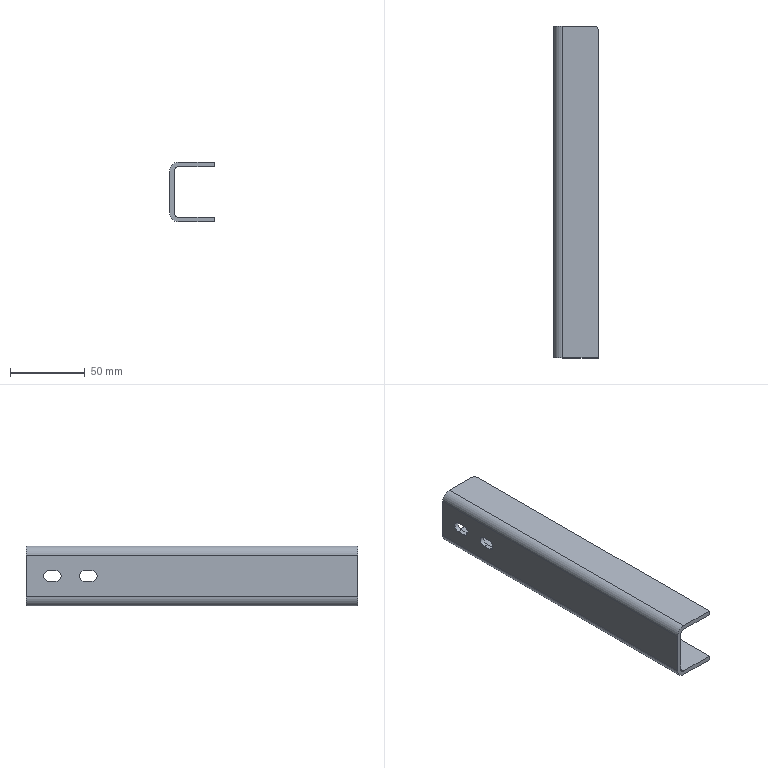Part | NX | features solid 2 | 1 solid | 24 faces | box 30 x 222 x 40 mm | volume 59579 mm3 | plane 14 | cylinder 10 | commonest cylinder face diameters 6 x4 7 x4 12 x2
STEP:
#1=CARTESIAN_POINT('',(340.,-413.,805.));
#2=VERTEX_POINT('',#1);
#3=CARTESIAN_POINT('',(343.,-416.,805.));
#4=VERTEX_POINT('',#3);
#5=CARTESIAN_POINT('',(340.,-416.,805.));
#6=DIRECTION('',(0.,0.,-1.));
#7=DIRECTION('',(-1.,0.,0.));
#8=AXIS2_PLACEMENT_3D('',#5,#6,#7);
#9=CIRCLE('',#8,3.);
#10=EDGE_CURVE('',#2,#4,#9,.T.);
#11=ORIENTED_EDGE('',*,*,#10,.F.);
#12=CARTESIAN_POINT('',(340.,-413.,808.));
#13=VERTEX_POINT('',#12);
#14=CARTESIAN_POINT('',(340.,-413.,802.));
#15=DIRECTION('',(0.,0.,-1.));
#16=VECTOR('',#15,1000.);
#17=LINE('',#14,#16);
#18=EDGE_CURVE('',#13,#2,#17,.T.);
#19=ORIENTED_EDGE('',*,*,#18,.F.);
#20=CARTESIAN_POINT('',(343.,-416.,808.));
#21=VERTEX_POINT('',#20);
#22=CARTESIAN_POINT('',(340.,-416.,808.));
#23=DIRECTION('',(0.,0.,1.));
#24=DIRECTION('',(-1.,0.,0.));
#25=AXIS2_PLACEMENT_3D('',#22,#23,#24);
#26=CIRCLE('',#25,3.);
#27=EDGE_CURVE('',#21,#13,#26,.T.);
#28=ORIENTED_EDGE('',*,*,#27,.F.);
#29=CARTESIAN_POINT('',(343.,-416.,808.));
#30=DIRECTION('',(0.,0.,1.));
#31=VECTOR('',#30,1000.);
#32=LINE('',#29,#31);
#33=EDGE_CURVE('',#4,#21,#32,.T.);
#34=ORIENTED_EDGE('',*,*,#33,.F.);
#35=EDGE_LOOP('',(#11,#19,#28,#34));
#36=FACE_BOUND('',#35,.T.);
#37=CARTESIAN_POINT('',(340.,-416.,808.));
#38=DIRECTION('',(0.,0.,1.));
#39=DIRECTION('',(1.,0.,0.));
#40=AXIS2_PLACEMENT_3D('',#37,#38,#39);
#41=CYLINDRICAL_SURFACE('',#40,3.);
#42=ADVANCED_FACE('',(#36),#41,.T.);
#43=CARTESIAN_POINT('',(343.,-416.,771.));
#44=VERTEX_POINT('',#43);
#45=CARTESIAN_POINT('',(340.,-413.,771.));
#46=VERTEX_POINT('',#45);
#47=CARTESIAN_POINT('',(340.,-416.,771.));
#48=DIRECTION('',(0.,0.,1.));
#49=DIRECTION('',(1.,0.,0.));
#50=AXIS2_PLACEMENT_3D('',#47,#48,#49);
#51=CIRCLE('',#50,3.);
#52=EDGE_CURVE('',#44,#46,#51,.T.);
#53=ORIENTED_EDGE('',*,*,#52,.F.);
#54=CARTESIAN_POINT('',(343.,-416.,768.));
#55=VERTEX_POINT('',#54);
#56=CARTESIAN_POINT('',(343.,-416.,768.));
#57=DIRECTION('',(0.,0.,1.));
#58=VECTOR('',#57,1000.);
#59=LINE('',#56,#58);
#60=EDGE_CURVE('',#55,#44,#59,.T.);
#61=ORIENTED_EDGE('',*,*,#60,.F.);
#62=CARTESIAN_POINT('',(340.,-413.,768.));
#63=VERTEX_POINT('',#62);
#64=CARTESIAN_POINT('',(340.,-416.,768.));
#65=DIRECTION('',(0.,0.,-1.));
#66=DIRECTION('',(1.,0.,0.));
#67=AXIS2_PLACEMENT_3D('',#64,#65,#66);
#68=CIRCLE('',#67,3.);
#69=EDGE_CURVE('',#63,#55,#68,.T.);
#70=ORIENTED_EDGE('',*,*,#69,.F.);
#71=CARTESIAN_POINT('',(340.,-413.,802.));
#72=DIRECTION('',(0.,0.,-1.));
#73=VECTOR('',#72,1000.);
#74=LINE('',#71,#73);
#75=EDGE_CURVE('',#46,#63,#74,.T.);
#76=ORIENTED_EDGE('',*,*,#75,.F.);
#77=EDGE_LOOP('',(#53,#61,#70,#76));
#78=FACE_BOUND('',#77,.T.);
#79=CARTESIAN_POINT('',(340.,-416.,802.));
#80=DIRECTION('',(0.,0.,1.));
#81=DIRECTION('',(1.,0.,0.));
#82=AXIS2_PLACEMENT_3D('',#79,#80,#81);
#83=CYLINDRICAL_SURFACE('',#82,3.);
#84=ADVANCED_FACE('',(#78),#83,.T.);
#85=CARTESIAN_POINT('',(313.,-428.,791.5));
#86=VERTEX_POINT('',#85);
#87=CARTESIAN_POINT('',(316.,-428.,791.5));
#88=VERTEX_POINT('',#87);
#89=CARTESIAN_POINT('',(88.439,-428.,791.5));
#90=DIRECTION('',(1.,0.,0.));
#91=VECTOR('',#90,1000.);
#92=LINE('',#89,#91);
#93=EDGE_CURVE('',#86,#88,#92,.T.);
#94=ORIENTED_EDGE('',*,*,#93,.T.);
#95=CARTESIAN_POINT('',(316.,-433.,791.5));
#96=VERTEX_POINT('',#95);
#97=CARTESIAN_POINT('',(316.,-428.,791.5));
#98=DIRECTION('',(0.,-1.,0.));
#99=VECTOR('',#98,1000.);
#100=LINE('',#97,#99);
#101=EDGE_CURVE('',#88,#96,#100,.T.);
#102=ORIENTED_EDGE('',*,*,#101,.T.);
#103=CARTESIAN_POINT('',(313.,-433.,791.5));
#104=VERTEX_POINT('',#103);
#105=CARTESIAN_POINT('',(88.439,-433.,791.5));
#106=DIRECTION('',(1.,0.,0.));
#107=VECTOR('',#106,1000.);
#108=LINE('',#105,#107);
#109=EDGE_CURVE('',#104,#96,#108,.T.);
#110=ORIENTED_EDGE('',*,*,#109,.F.);
#111=CARTESIAN_POINT('',(313.,-635.,791.5));
#112=DIRECTION('',(0.,-1.,0.));
#113=VECTOR('',#112,1000.);
#114=LINE('',#111,#113);
#115=EDGE_CURVE('',#86,#104,#114,.T.);
#116=ORIENTED_EDGE('',*,*,#115,.F.);
#117=EDGE_LOOP('',(#94,#102,#110,#116));
#118=FACE_BOUND('',#117,.T.);
#119=CARTESIAN_POINT('',(88.439,-428.,791.5));
#120=DIRECTION('',(0.,0.,1.));
#121=DIRECTION('',(0.,-1.,0.));
#122=AXIS2_PLACEMENT_3D('',#119,#120,#121);
#123=PLANE('',#122);
#124=ADVANCED_FACE('',(#118),#123,.F.);
#125=CARTESIAN_POINT('',(313.,-428.,784.5));
#126=VERTEX_POINT('',#125);
#127=CARTESIAN_POINT('',(316.,-428.,784.5));
#128=VERTEX_POINT('',#127);
#129=CARTESIAN_POINT('',(88.439,-428.,784.5));
#130=DIRECTION('',(1.,0.,0.));
#131=VECTOR('',#130,1000.);
#132=LINE('',#129,#131);
#133=EDGE_CURVE('',#126,#128,#132,.T.);
#134=ORIENTED_EDGE('',*,*,#133,.T.);
#135=CARTESIAN_POINT('',(316.,-428.,788.));
#136=DIRECTION('',(1.,0.,0.));
#137=DIRECTION('',(0.,-1.,0.));
#138=AXIS2_PLACEMENT_3D('',#135,#136,#137);
#139=CIRCLE('',#138,3.5);
#140=EDGE_CURVE('',#128,#88,#139,.T.);
#141=ORIENTED_EDGE('',*,*,#140,.T.);
#142=ORIENTED_EDGE('',*,*,#93,.F.);
#143=CARTESIAN_POINT('',(313.,-428.,788.));
#144=DIRECTION('',(1.,0.,0.));
#145=DIRECTION('',(0.,0.,-1.));
#146=AXIS2_PLACEMENT_3D('',#143,#144,#145);
#147=CIRCLE('',#146,3.5);
#148=EDGE_CURVE('',#126,#86,#147,.T.);
#149=ORIENTED_EDGE('',*,*,#148,.F.);
#150=EDGE_LOOP('',(#134,#141,#142,#149));
#151=FACE_BOUND('',#150,.T.);
#152=CARTESIAN_POINT('',(88.439,-428.,788.));
#153=DIRECTION('',(1.,0.,0.));
#154=DIRECTION('',(0.,0.,-1.));
#155=AXIS2_PLACEMENT_3D('',#152,#153,#154);
#156=CYLINDRICAL_SURFACE('',#155,3.5);
#157=ADVANCED_FACE('',(#151),#156,.F.);
#158=CARTESIAN_POINT('',(313.,-433.,784.5));
#159=VERTEX_POINT('',#158);
#160=CARTESIAN_POINT('',(316.,-433.,784.5));
#161=VERTEX_POINT('',#160);
#162=CARTESIAN_POINT('',(88.439,-433.,784.5));
#163=DIRECTION('',(1.,0.,0.));
#164=VECTOR('',#163,1000.);
#165=LINE('',#162,#164);
#166=EDGE_CURVE('',#159,#161,#165,.T.);
#167=ORIENTED_EDGE('',*,*,#166,.T.);
#168=CARTESIAN_POINT('',(316.,-428.,784.5));
#169=DIRECTION('',(0.,1.,0.));
#170=VECTOR('',#169,1000.);
#171=LINE('',#168,#170);
#172=EDGE_CURVE('',#161,#128,#171,.T.);
#173=ORIENTED_EDGE('',*,*,#172,.T.);
#174=ORIENTED_EDGE('',*,*,#133,.F.);
#175=CARTESIAN_POINT('',(313.,-635.,784.5));
#176=DIRECTION('',(0.,1.,0.));
#177=VECTOR('',#176,1000.);
#178=LINE('',#175,#177);
#179=EDGE_CURVE('',#159,#126,#178,.T.);
#180=ORIENTED_EDGE('',*,*,#179,.F.);
#181=EDGE_LOOP('',(#167,#173,#174,#180));
#182=FACE_BOUND('',#181,.T.);
#183=CARTESIAN_POINT('',(88.439,-428.,784.5));
#184=DIRECTION('',(0.,0.,-1.));
#185=DIRECTION('',(-1.,0.,0.));
#186=AXIS2_PLACEMENT_3D('',#183,#184,#185);
#187=PLANE('',#186);
#188=ADVANCED_FACE('',(#182),#187,.F.);
#189=ORIENTED_EDGE('',*,*,#109,.T.);
#190=CARTESIAN_POINT('',(316.,-433.,788.));
#191=DIRECTION('',(1.,0.,0.));
#192=DIRECTION('',(0.,1.,0.));
#193=AXIS2_PLACEMENT_3D('',#190,#191,#192);
#194=CIRCLE('',#193,3.5);
#195=EDGE_CURVE('',#96,#161,#194,.T.);
#196=ORIENTED_EDGE('',*,*,#195,.T.);
#197=ORIENTED_EDGE('',*,*,#166,.F.);
#198=CARTESIAN_POINT('',(313.,-433.,788.));
#199=DIRECTION('',(1.,0.,0.));
#200=DIRECTION('',(0.,0.,-1.));
#201=AXIS2_PLACEMENT_3D('',#198,#199,#200);
#202=CIRCLE('',#201,3.5);
#203=EDGE_CURVE('',#104,#159,#202,.T.);
#204=ORIENTED_EDGE('',*,*,#203,.F.);
#205=EDGE_LOOP('',(#189,#196,#197,#204));
#206=FACE_BOUND('',#205,.T.);
#207=CARTESIAN_POINT('',(88.439,-433.,788.));
#208=DIRECTION('',(1.,0.,0.));
#209=DIRECTION('',(0.,0.,-1.));
#210=AXIS2_PLACEMENT_3D('',#207,#208,#209);
#211=CYLINDRICAL_SURFACE('',#210,3.5);
#212=ADVANCED_FACE('',(#206),#211,.F.);
#213=CARTESIAN_POINT('',(313.,-452.,791.5));
#214=VERTEX_POINT('',#213);
#215=CARTESIAN_POINT('',(316.,-452.,791.5));
#216=VERTEX_POINT('',#215);
#217=CARTESIAN_POINT('',(88.439,-452.,791.5));
#218=DIRECTION('',(1.,0.,0.));
#219=VECTOR('',#218,1000.);
#220=LINE('',#217,#219);
#221=EDGE_CURVE('',#214,#216,#220,.T.);
#222=ORIENTED_EDGE('',*,*,#221,.T.);
#223=CARTESIAN_POINT('',(316.,-457.,791.5));
#224=VERTEX_POINT('',#223);
#225=CARTESIAN_POINT('',(316.,-452.,791.5));
#226=DIRECTION('',(0.,-1.,0.));
#227=VECTOR('',#226,1000.);
#228=LINE('',#225,#227);
#229=EDGE_CURVE('',#216,#224,#228,.T.);
#230=ORIENTED_EDGE('',*,*,#229,.T.);
#231=CARTESIAN_POINT('',(313.,-457.,791.5));
#232=VERTEX_POINT('',#231);
#233=CARTESIAN_POINT('',(88.439,-457.,791.5));
#234=DIRECTION('',(1.,0.,0.));
#235=VECTOR('',#234,1000.);
#236=LINE('',#233,#235);
#237=EDGE_CURVE('',#232,#224,#236,.T.);
#238=ORIENTED_EDGE('',*,*,#237,.F.);
#239=CARTESIAN_POINT('',(313.,-635.,791.5));
#240=DIRECTION('',(0.,-1.,0.));
#241=VECTOR('',#240,1000.);
#242=LINE('',#239,#241);
#243=EDGE_CURVE('',#214,#232,#242,.T.);
#244=ORIENTED_EDGE('',*,*,#243,.F.);
#245=EDGE_LOOP('',(#222,#230,#238,#244));
#246=FACE_BOUND('',#245,.T.);
#247=CARTESIAN_POINT('',(88.439,-452.,791.5));
#248=DIRECTION('',(0.,0.,1.));
#249=DIRECTION('',(0.,-1.,0.));
#250=AXIS2_PLACEMENT_3D('',#247,#248,#249);
#251=PLANE('',#250);
#252=ADVANCED_FACE('',(#246),#251,.F.);
#253=CARTESIAN_POINT('',(313.,-452.,784.5));
#254=VERTEX_POINT('',#253);
#255=CARTESIAN_POINT('',(316.,-452.,784.5));
#256=VERTEX_POINT('',#255);
#257=CARTESIAN_POINT('',(88.439,-452.,784.5));
#258=DIRECTION('',(1.,0.,0.));
#259=VECTOR('',#258,1000.);
#260=LINE('',#257,#259);
#261=EDGE_CURVE('',#254,#256,#260,.T.);
#262=ORIENTED_EDGE('',*,*,#261,.T.);
#263=CARTESIAN_POINT('',(316.,-452.,788.));
#264=DIRECTION('',(1.,0.,0.));
#265=DIRECTION('',(0.,-1.,0.));
#266=AXIS2_PLACEMENT_3D('',#263,#264,#265);
#267=CIRCLE('',#266,3.5);
#268=EDGE_CURVE('',#256,#216,#267,.T.);
#269=ORIENTED_EDGE('',*,*,#268,.T.);
#270=ORIENTED_EDGE('',*,*,#221,.F.);
#271=CARTESIAN_POINT('',(313.,-452.,788.));
#272=DIRECTION('',(1.,0.,0.));
#273=DIRECTION('',(0.,0.,-1.));
#274=AXIS2_PLACEMENT_3D('',#271,#272,#273);
#275=CIRCLE('',#274,3.5);
#276=EDGE_CURVE('',#254,#214,#275,.T.);
#277=ORIENTED_EDGE('',*,*,#276,.F.);
#278=EDGE_LOOP('',(#262,#269,#270,#277));
#279=FACE_BOUND('',#278,.T.);
#280=CARTESIAN_POINT('',(88.439,-452.,788.));
#281=DIRECTION('',(1.,0.,0.));
#282=DIRECTION('',(0.,0.,-1.));
#283=AXIS2_PLACEMENT_3D('',#280,#281,#282);
#284=CYLINDRICAL_SURFACE('',#283,3.5);
#285=ADVANCED_FACE('',(#279),#284,.F.);
#286=CARTESIAN_POINT('',(313.,-457.,784.5));
#287=VERTEX_POINT('',#286);
#288=CARTESIAN_POINT('',(316.,-457.,784.5));
#289=VERTEX_POINT('',#288);
#290=CARTESIAN_POINT('',(88.439,-457.,784.5));
#291=DIRECTION('',(1.,0.,0.));
#292=VECTOR('',#291,1000.);
#293=LINE('',#290,#292);
#294=EDGE_CURVE('',#287,#289,#293,.T.);
#295=ORIENTED_EDGE('',*,*,#294,.T.);
#296=CARTESIAN_POINT('',(316.,-452.,784.5));
#297=DIRECTION('',(0.,1.,0.));
#298=VECTOR('',#297,1000.);
#299=LINE('',#296,#298);
#300=EDGE_CURVE('',#289,#256,#299,.T.);
#301=ORIENTED_EDGE('',*,*,#300,.T.);
#302=ORIENTED_EDGE('',*,*,#261,.F.);
#303=CARTESIAN_POINT('',(313.,-635.,784.5));
#304=DIRECTION('',(0.,1.,0.));
#305=VECTOR('',#304,1000.);
#306=LINE('',#303,#305);
#307=EDGE_CURVE('',#287,#254,#306,.T.);
#308=ORIENTED_EDGE('',*,*,#307,.F.);
#309=EDGE_LOOP('',(#295,#301,#302,#308));
#310=FACE_BOUND('',#309,.T.);
#311=CARTESIAN_POINT('',(88.439,-452.,784.5));
#312=DIRECTION('',(0.,0.,-1.));
#313=DIRECTION('',(-1.,0.,0.));
#314=AXIS2_PLACEMENT_3D('',#311,#312,#313);
#315=PLANE('',#314);
#316=ADVANCED_FACE('',(#310),#315,.F.);
#317=ORIENTED_EDGE('',*,*,#237,.T.);
#318=CARTESIAN_POINT('',(316.,-457.,788.));
#319=DIRECTION('',(1.,0.,0.));
#320=DIRECTION('',(0.,1.,0.));
#321=AXIS2_PLACEMENT_3D('',#318,#319,#320);
#322=CIRCLE('',#321,3.5);
#323=EDGE_CURVE('',#224,#289,#322,.T.);
#324=ORIENTED_EDGE('',*,*,#323,.T.);
#325=ORIENTED_EDGE('',*,*,#294,.F.);
#326=CARTESIAN_POINT('',(313.,-457.,788.));
#327=DIRECTION('',(1.,0.,0.));
#328=DIRECTION('',(0.,0.,-1.));
#329=AXIS2_PLACEMENT_3D('',#326,#327,#328);
#330=CIRCLE('',#329,3.5);
#331=EDGE_CURVE('',#232,#287,#330,.T.);
#332=ORIENTED_EDGE('',*,*,#331,.F.);
#333=EDGE_LOOP('',(#317,#324,#325,#332));
#334=FACE_BOUND('',#333,.T.);
#335=CARTESIAN_POINT('',(88.439,-457.,788.));
#336=DIRECTION('',(1.,0.,0.));
#337=DIRECTION('',(0.,0.,-1.));
#338=AXIS2_PLACEMENT_3D('',#335,#336,#337);
#339=CYLINDRICAL_SURFACE('',#338,3.5);
#340=ADVANCED_FACE('',(#334),#339,.F.);
#341=CARTESIAN_POINT('',(343.,-635.,771.));
#342=VERTEX_POINT('',#341);
#343=CARTESIAN_POINT('',(343.,-635.,771.));
#344=DIRECTION('',(0.,1.,0.));
#345=VECTOR('',#344,1000.);
#346=LINE('',#343,#345);
#347=EDGE_CURVE('',#342,#44,#346,.T.);
#348=ORIENTED_EDGE('',*,*,#347,.T.);
#349=ORIENTED_EDGE('',*,*,#52,.T.);
#350=CARTESIAN_POINT('',(319.,-413.,771.));
#351=VERTEX_POINT('',#350);
#352=CARTESIAN_POINT('',(313.,-413.,771.));
#353=DIRECTION('',(1.,0.,0.));
#354=VECTOR('',#353,1000.);
#355=LINE('',#352,#354);
#356=EDGE_CURVE('',#351,#46,#355,.T.);
#357=ORIENTED_EDGE('',*,*,#356,.F.);
#358=CARTESIAN_POINT('',(319.,-635.,771.));
#359=VERTEX_POINT('',#358);
#360=CARTESIAN_POINT('',(319.,-635.,771.));
#361=DIRECTION('',(0.,1.,0.));
#362=VECTOR('',#361,1000.);
#363=LINE('',#360,#362);
#364=EDGE_CURVE('',#359,#351,#363,.T.);
#365=ORIENTED_EDGE('',*,*,#364,.F.);
#366=CARTESIAN_POINT('',(313.,-635.,771.));
#367=DIRECTION('',(1.,0.,0.));
#368=VECTOR('',#367,1000.);
#369=LINE('',#366,#368);
#370=EDGE_CURVE('',#359,#342,#369,.T.);
#371=ORIENTED_EDGE('',*,*,#370,.T.);
#372=EDGE_LOOP('',(#348,#349,#357,#365,#371));
#373=FACE_BOUND('',#372,.T.);
#374=CARTESIAN_POINT('',(313.,-635.,771.));
#375=DIRECTION('',(0.,0.,1.));
#376=DIRECTION('',(1.,0.,0.));
#377=AXIS2_PLACEMENT_3D('',#374,#375,#376);
#378=PLANE('',#377);
#379=ADVANCED_FACE('',(#373),#378,.T.);
#380=CARTESIAN_POINT('',(316.,-413.,774.));
#381=VERTEX_POINT('',#380);
#382=CARTESIAN_POINT('',(319.,-413.,774.));
#383=DIRECTION('',(0.,-1.,0.));
#384=DIRECTION('',(0.,0.,1.));
#385=AXIS2_PLACEMENT_3D('',#382,#383,#384);
#386=CIRCLE('',#385,3.);
#387=EDGE_CURVE('',#381,#351,#386,.T.);
#388=ORIENTED_EDGE('',*,*,#387,.F.);
#389=CARTESIAN_POINT('',(316.,-635.,774.));
#390=VERTEX_POINT('',#389);
#391=CARTESIAN_POINT('',(316.,-635.,774.));
#392=DIRECTION('',(0.,1.,0.));
#393=VECTOR('',#392,1000.);
#394=LINE('',#391,#393);
#395=EDGE_CURVE('',#390,#381,#394,.T.);
#396=ORIENTED_EDGE('',*,*,#395,.F.);
#397=CARTESIAN_POINT('',(319.,-635.,774.));
#398=DIRECTION('',(0.,-1.,0.));
#399=DIRECTION('',(0.,0.,1.));
#400=AXIS2_PLACEMENT_3D('',#397,#398,#399);
#401=CIRCLE('',#400,3.);
#402=EDGE_CURVE('',#390,#359,#401,.T.);
#403=ORIENTED_EDGE('',*,*,#402,.T.);
#404=ORIENTED_EDGE('',*,*,#364,.T.);
#405=EDGE_LOOP('',(#388,#396,#403,#404));
#406=FACE_BOUND('',#405,.T.);
#407=CARTESIAN_POINT('',(319.,-635.,774.));
#408=DIRECTION('',(0.,1.,0.));
#409=DIRECTION('',(0.,0.,1.));
#410=AXIS2_PLACEMENT_3D('',#407,#408,#409);
#411=CYLINDRICAL_SURFACE('',#410,3.);
#412=ADVANCED_FACE('',(#406),#411,.F.);
#413=ORIENTED_EDGE('',*,*,#323,.F.);
#414=ORIENTED_EDGE('',*,*,#229,.F.);
#415=ORIENTED_EDGE('',*,*,#268,.F.);
#416=ORIENTED_EDGE('',*,*,#300,.F.);
#417=EDGE_LOOP('',(#413,#414,#415,#416));
#418=FACE_BOUND('',#417,.T.);
#419=ORIENTED_EDGE('',*,*,#195,.F.);
#420=ORIENTED_EDGE('',*,*,#101,.F.);
#421=ORIENTED_EDGE('',*,*,#140,.F.);
#422=ORIENTED_EDGE('',*,*,#172,.F.);
#423=EDGE_LOOP('',(#419,#420,#421,#422));
#424=FACE_BOUND('',#423,.T.);
#425=CARTESIAN_POINT('',(316.,-413.,802.));
#426=VERTEX_POINT('',#425);
#427=CARTESIAN_POINT('',(316.,-413.,808.));
#428=DIRECTION('',(0.,0.,-1.));
#429=VECTOR('',#428,1000.);
#430=LINE('',#427,#429);
#431=EDGE_CURVE('',#426,#381,#430,.T.);
#432=ORIENTED_EDGE('',*,*,#431,.F.);
#433=CARTESIAN_POINT('',(316.,-635.,802.));
#434=VERTEX_POINT('',#433);
#435=CARTESIAN_POINT('',(316.,-635.,802.));
#436=DIRECTION('',(0.,1.,0.));
#437=VECTOR('',#436,1000.);
#438=LINE('',#435,#437);
#439=EDGE_CURVE('',#434,#426,#438,.T.);
#440=ORIENTED_EDGE('',*,*,#439,.F.);
#441=CARTESIAN_POINT('',(316.,-635.,808.));
#442=DIRECTION('',(0.,0.,-1.));
#443=VECTOR('',#442,1000.);
#444=LINE('',#441,#443);
#445=EDGE_CURVE('',#434,#390,#444,.T.);
#446=ORIENTED_EDGE('',*,*,#445,.T.);
#447=ORIENTED_EDGE('',*,*,#395,.T.);
#448=EDGE_LOOP('',(#432,#440,#446,#447));
#449=FACE_BOUND('',#448,.T.);
#450=CARTESIAN_POINT('',(316.,-635.,808.));
#451=DIRECTION('',(1.,0.,0.));
#452=DIRECTION('',(0.,1.,0.));
#453=AXIS2_PLACEMENT_3D('',#450,#451,#452);
#454=PLANE('',#453);
#455=ADVANCED_FACE('',(#418,#424,#449),#454,.T.);
#456=CARTESIAN_POINT('',(319.,-413.,805.));
#457=VERTEX_POINT('',#456);
#458=CARTESIAN_POINT('',(319.,-413.,802.));
#459=DIRECTION('',(0.,-1.,0.));
#460=DIRECTION('',(0.,0.,1.));
#461=AXIS2_PLACEMENT_3D('',#458,#459,#460);
#462=CIRCLE('',#461,3.);
#463=EDGE_CURVE('',#457,#426,#462,.T.);
#464=ORIENTED_EDGE('',*,*,#463,.F.);
#465=CARTESIAN_POINT('',(319.,-635.,805.));
#466=VERTEX_POINT('',#465);
#467=CARTESIAN_POINT('',(319.,-635.,805.));
#468=DIRECTION('',(0.,1.,0.));
#469=VECTOR('',#468,1000.);
#470=LINE('',#467,#469);
#471=EDGE_CURVE('',#466,#457,#470,.T.);
#472=ORIENTED_EDGE('',*,*,#471,.F.);
#473=CARTESIAN_POINT('',(319.,-635.,802.));
#474=DIRECTION('',(0.,-1.,0.));
#475=DIRECTION('',(0.,0.,1.));
#476=AXIS2_PLACEMENT_3D('',#473,#474,#475);
#477=CIRCLE('',#476,3.);
#478=EDGE_CURVE('',#466,#434,#477,.T.);
#479=ORIENTED_EDGE('',*,*,#478,.T.);
#480=ORIENTED_EDGE('',*,*,#439,.T.);
#481=EDGE_LOOP('',(#464,#472,#479,#480));
#482=FACE_BOUND('',#481,.T.);
#483=CARTESIAN_POINT('',(319.,-635.,802.));
#484=DIRECTION('',(0.,1.,0.));
#485=DIRECTION('',(0.,0.,1.));
#486=AXIS2_PLACEMENT_3D('',#483,#484,#485);
#487=CYLINDRICAL_SURFACE('',#486,3.);
#488=ADVANCED_FACE('',(#482),#487,.F.);
#489=CARTESIAN_POINT('',(343.,-413.,805.));
#490=DIRECTION('',(-1.,0.,0.));
#491=VECTOR('',#490,1000.);
#492=LINE('',#489,#491);
#493=EDGE_CURVE('',#2,#457,#492,.T.);
#494=ORIENTED_EDGE('',*,*,#493,.F.);
#495=ORIENTED_EDGE('',*,*,#10,.T.);
#496=CARTESIAN_POINT('',(343.,-635.,805.));
#497=VERTEX_POINT('',#496);
#498=CARTESIAN_POINT('',(343.,-635.,805.));
#499=DIRECTION('',(0.,1.,0.));
#500=VECTOR('',#499,1000.);
#501=LINE('',#498,#500);
#502=EDGE_CURVE('',#497,#4,#501,.T.);
#503=ORIENTED_EDGE('',*,*,#502,.F.);
#504=CARTESIAN_POINT('',(343.,-635.,805.));
#505=DIRECTION('',(-1.,0.,0.));
#506=VECTOR('',#505,1000.);
#507=LINE('',#504,#506);
#508=EDGE_CURVE('',#497,#466,#507,.T.);
#509=ORIENTED_EDGE('',*,*,#508,.T.);
#510=ORIENTED_EDGE('',*,*,#471,.T.);
#511=EDGE_LOOP('',(#494,#495,#503,#509,#510));
#512=FACE_BOUND('',#511,.T.);
#513=CARTESIAN_POINT('',(343.,-635.,805.));
#514=DIRECTION('',(0.,0.,-1.));
#515=DIRECTION('',(0.,-1.,0.));
#516=AXIS2_PLACEMENT_3D('',#513,#514,#515);
#517=PLANE('',#516);
#518=ADVANCED_FACE('',(#512),#517,.T.);
#519=CARTESIAN_POINT('',(319.,-413.,768.));
#520=VERTEX_POINT('',#519);
#521=CARTESIAN_POINT('',(313.,-413.,768.));
#522=DIRECTION('',(1.,0.,0.));
#523=VECTOR('',#522,1000.);
#524=LINE('',#521,#523);
#525=EDGE_CURVE('',#520,#63,#524,.T.);
#526=ORIENTED_EDGE('',*,*,#525,.T.);
#527=ORIENTED_EDGE('',*,*,#69,.T.);
#528=CARTESIAN_POINT('',(343.,-635.,768.));
#529=VERTEX_POINT('',#528);
#530=CARTESIAN_POINT('',(343.,-635.,768.));
#531=DIRECTION('',(0.,1.,0.));
#532=VECTOR('',#531,1000.);
#533=LINE('',#530,#532);
#534=EDGE_CURVE('',#529,#55,#533,.T.);
#535=ORIENTED_EDGE('',*,*,#534,.F.);
#536=CARTESIAN_POINT('',(319.,-635.,768.));
#537=VERTEX_POINT('',#536);
#538=CARTESIAN_POINT('',(313.,-635.,768.));
#539=DIRECTION('',(1.,0.,0.));
#540=VECTOR('',#539,1000.);
#541=LINE('',#538,#540);
#542=EDGE_CURVE('',#537,#529,#541,.T.);
#543=ORIENTED_EDGE('',*,*,#542,.F.);
#544=CARTESIAN_POINT('',(319.,-635.,768.));
#545=DIRECTION('',(0.,1.,0.));
#546=VECTOR('',#545,1000.);
#547=LINE('',#544,#546);
#548=EDGE_CURVE('',#537,#520,#547,.T.);
#549=ORIENTED_EDGE('',*,*,#548,.T.);
#550=EDGE_LOOP('',(#526,#527,#535,#543,#549));
#551=FACE_BOUND('',#550,.T.);
#552=CARTESIAN_POINT('',(313.,-635.,768.));
#553=DIRECTION('',(0.,0.,1.));
#554=DIRECTION('',(1.,0.,0.));
#555=AXIS2_PLACEMENT_3D('',#552,#553,#554);
#556=PLANE('',#555);
#557=ADVANCED_FACE('',(#551),#556,.F.);
#558=CARTESIAN_POINT('',(313.,-413.,774.));
#559=VERTEX_POINT('',#558);
#560=CARTESIAN_POINT('',(319.,-413.,774.));
#561=DIRECTION('',(0.,-1.,0.));
#562=DIRECTION('',(0.,0.,1.));
#563=AXIS2_PLACEMENT_3D('',#560,#561,#562);
#564=CIRCLE('',#563,6.);
#565=EDGE_CURVE('',#559,#520,#564,.T.);
#566=ORIENTED_EDGE('',*,*,#565,.T.);
#567=ORIENTED_EDGE('',*,*,#548,.F.);
#568=CARTESIAN_POINT('',(313.,-635.,774.));
#569=VERTEX_POINT('',#568);
#570=CARTESIAN_POINT('',(319.,-635.,774.));
#571=DIRECTION('',(0.,-1.,0.));
#572=DIRECTION('',(0.,0.,1.));
#573=AXIS2_PLACEMENT_3D('',#570,#571,#572);
#574=CIRCLE('',#573,6.);
#575=EDGE_CURVE('',#569,#537,#574,.T.);
#576=ORIENTED_EDGE('',*,*,#575,.F.);
#577=CARTESIAN_POINT('',(313.,-635.,774.));
#578=DIRECTION('',(0.,1.,0.));
#579=VECTOR('',#578,1000.);
#580=LINE('',#577,#579);
#581=EDGE_CURVE('',#569,#559,#580,.T.);
#582=ORIENTED_EDGE('',*,*,#581,.T.);
#583=EDGE_LOOP('',(#566,#567,#576,#582));
#584=FACE_BOUND('',#583,.T.);
#585=CARTESIAN_POINT('',(319.,-635.,774.));
#586=DIRECTION('',(0.,1.,0.));
#587=DIRECTION('',(0.,0.,1.));
#588=AXIS2_PLACEMENT_3D('',#585,#586,#587);
#589=CYLINDRICAL_SURFACE('',#588,6.);
#590=ADVANCED_FACE('',(#584),#589,.T.);
#591=ORIENTED_EDGE('',*,*,#243,.T.);
#592=ORIENTED_EDGE('',*,*,#331,.T.);
#593=ORIENTED_EDGE('',*,*,#307,.T.);
#594=ORIENTED_EDGE('',*,*,#276,.T.);
#595=EDGE_LOOP('',(#591,#592,#593,#594));
#596=FACE_BOUND('',#595,.T.);
#597=ORIENTED_EDGE('',*,*,#115,.T.);
#598=ORIENTED_EDGE('',*,*,#203,.T.);
#599=ORIENTED_EDGE('',*,*,#179,.T.);
#600=ORIENTED_EDGE('',*,*,#148,.T.);
#601=EDGE_LOOP('',(#597,#598,#599,#600));
#602=FACE_BOUND('',#601,.T.);
#603=CARTESIAN_POINT('',(313.,-413.,802.));
#604=VERTEX_POINT('',#603);
#605=CARTESIAN_POINT('',(313.,-413.,808.));
#606=DIRECTION('',(0.,0.,-1.));
#607=VECTOR('',#606,1000.);
#608=LINE('',#605,#607);
#609=EDGE_CURVE('',#604,#559,#608,.T.);
#610=ORIENTED_EDGE('',*,*,#609,.T.);
#611=ORIENTED_EDGE('',*,*,#581,.F.);
#612=CARTESIAN_POINT('',(313.,-635.,802.));
#613=VERTEX_POINT('',#612);
#614=CARTESIAN_POINT('',(313.,-635.,808.));
#615=DIRECTION('',(0.,0.,-1.));
#616=VECTOR('',#615,1000.);
#617=LINE('',#614,#616);
#618=EDGE_CURVE('',#613,#569,#617,.T.);
#619=ORIENTED_EDGE('',*,*,#618,.F.);
#620=CARTESIAN_POINT('',(313.,-635.,802.));
#621=DIRECTION('',(0.,1.,0.));
#622=VECTOR('',#621,1000.);
#623=LINE('',#620,#622);
#624=EDGE_CURVE('',#613,#604,#623,.T.);
#625=ORIENTED_EDGE('',*,*,#624,.T.);
#626=EDGE_LOOP('',(#610,#611,#619,#625));
#627=FACE_BOUND('',#626,.T.);
#628=CARTESIAN_POINT('',(313.,-635.,808.));
#629=DIRECTION('',(1.,0.,0.));
#630=DIRECTION('',(0.,1.,0.));
#631=AXIS2_PLACEMENT_3D('',#628,#629,#630);
#632=PLANE('',#631);
#633=ADVANCED_FACE('',(#596,#602,#627),#632,.F.);
#634=CARTESIAN_POINT('',(319.,-413.,808.));
#635=VERTEX_POINT('',#634);
#636=CARTESIAN_POINT('',(319.,-413.,802.));
#637=DIRECTION('',(0.,-1.,0.));
#638=DIRECTION('',(0.,0.,1.));
#639=AXIS2_PLACEMENT_3D('',#636,#637,#638);
#640=CIRCLE('',#639,6.);
#641=EDGE_CURVE('',#635,#604,#640,.T.);
#642=ORIENTED_EDGE('',*,*,#641,.T.);
#643=ORIENTED_EDGE('',*,*,#624,.F.);
#644=CARTESIAN_POINT('',(319.,-635.,808.));
#645=VERTEX_POINT('',#644);
#646=CARTESIAN_POINT('',(319.,-635.,802.));
#647=DIRECTION('',(0.,-1.,0.));
#648=DIRECTION('',(0.,0.,1.));
#649=AXIS2_PLACEMENT_3D('',#646,#647,#648);
#650=CIRCLE('',#649,6.);
#651=EDGE_CURVE('',#645,#613,#650,.T.);
#652=ORIENTED_EDGE('',*,*,#651,.F.);
#653=CARTESIAN_POINT('',(319.,-635.,808.));
#654=DIRECTION('',(0.,1.,0.));
#655=VECTOR('',#654,1000.);
#656=LINE('',#653,#655);
#657=EDGE_CURVE('',#645,#635,#656,.T.);
#658=ORIENTED_EDGE('',*,*,#657,.T.);
#659=EDGE_LOOP('',(#642,#643,#652,#658));
#660=FACE_BOUND('',#659,.T.);
#661=CARTESIAN_POINT('',(319.,-635.,802.));
#662=DIRECTION('',(0.,1.,0.));
#663=DIRECTION('',(0.,0.,1.));
#664=AXIS2_PLACEMENT_3D('',#661,#662,#663);
#665=CYLINDRICAL_SURFACE('',#664,6.);
#666=ADVANCED_FACE('',(#660),#665,.T.);
#667=CARTESIAN_POINT('',(343.,-635.,808.));
#668=VERTEX_POINT('',#667);
#669=CARTESIAN_POINT('',(343.,-635.,808.));
#670=DIRECTION('',(0.,1.,0.));
#671=VECTOR('',#670,1000.);
#672=LINE('',#669,#671);
#673=EDGE_CURVE('',#668,#21,#672,.T.);
#674=ORIENTED_EDGE('',*,*,#673,.T.);
#675=ORIENTED_EDGE('',*,*,#27,.T.);
#676=CARTESIAN_POINT('',(343.,-413.,808.));
#677=DIRECTION('',(-1.,0.,0.));
#678=VECTOR('',#677,1000.);
#679=LINE('',#676,#678);
#680=EDGE_CURVE('',#13,#635,#679,.T.);
#681=ORIENTED_EDGE('',*,*,#680,.T.);
#682=ORIENTED_EDGE('',*,*,#657,.F.);
#683=CARTESIAN_POINT('',(343.,-635.,808.));
#684=DIRECTION('',(-1.,0.,0.));
#685=VECTOR('',#684,1000.);
#686=LINE('',#683,#685);
#687=EDGE_CURVE('',#668,#645,#686,.T.);
#688=ORIENTED_EDGE('',*,*,#687,.F.);
#689=EDGE_LOOP('',(#674,#675,#681,#682,#688));
#690=FACE_BOUND('',#689,.T.);
#691=CARTESIAN_POINT('',(343.,-635.,808.));
#692=DIRECTION('',(0.,0.,-1.));
#693=DIRECTION('',(0.,-1.,0.));
#694=AXIS2_PLACEMENT_3D('',#691,#692,#693);
#695=PLANE('',#694);
#696=ADVANCED_FACE('',(#690),#695,.F.);
#697=ORIENTED_EDGE('',*,*,#356,.T.);
#698=ORIENTED_EDGE('',*,*,#75,.T.);
#699=ORIENTED_EDGE('',*,*,#525,.F.);
#700=ORIENTED_EDGE('',*,*,#565,.F.);
#701=ORIENTED_EDGE('',*,*,#609,.F.);
#702=ORIENTED_EDGE('',*,*,#641,.F.);
#703=ORIENTED_EDGE('',*,*,#680,.F.);
#704=ORIENTED_EDGE('',*,*,#18,.T.);
#705=ORIENTED_EDGE('',*,*,#493,.T.);
#706=ORIENTED_EDGE('',*,*,#463,.T.);
#707=ORIENTED_EDGE('',*,*,#431,.T.);
#708=ORIENTED_EDGE('',*,*,#387,.T.);
#709=EDGE_LOOP('',(#697,#698,#699,#700,#701,#702,#703,#704,#705,#706,#707,#708));
#710=FACE_BOUND('',#709,.T.);
#711=CARTESIAN_POINT('',(319.,-413.,802.));
#712=DIRECTION('',(0.,-1.,0.));
#713=DIRECTION('',(0.,0.,-1.));
#714=AXIS2_PLACEMENT_3D('',#711,#712,#713);
#715=PLANE('',#714);
#716=ADVANCED_FACE('',(#710),#715,.F.);
#717=ORIENTED_EDGE('',*,*,#502,.T.);
#718=ORIENTED_EDGE('',*,*,#33,.T.);
#719=ORIENTED_EDGE('',*,*,#673,.F.);
#720=CARTESIAN_POINT('',(343.,-635.,808.));
#721=DIRECTION('',(0.,0.,1.));
#722=VECTOR('',#721,1000.);
#723=LINE('',#720,#722);
#724=EDGE_CURVE('',#497,#668,#723,.T.);
#725=ORIENTED_EDGE('',*,*,#724,.F.);
#726=EDGE_LOOP('',(#717,#718,#719,#725));
#727=FACE_BOUND('',#726,.T.);
#728=CARTESIAN_POINT('',(343.,-635.,808.));
#729=DIRECTION('',(-1.,0.,0.));
#730=DIRECTION('',(0.,0.,1.));
#731=AXIS2_PLACEMENT_3D('',#728,#729,#730);
#732=PLANE('',#731);
#733=ADVANCED_FACE('',(#727),#732,.F.);
#734=ORIENTED_EDGE('',*,*,#687,.T.);
#735=ORIENTED_EDGE('',*,*,#651,.T.);
#736=ORIENTED_EDGE('',*,*,#618,.T.);
#737=ORIENTED_EDGE('',*,*,#575,.T.);
#738=ORIENTED_EDGE('',*,*,#542,.T.);
#739=CARTESIAN_POINT('',(343.,-635.,768.));
#740=DIRECTION('',(0.,0.,-1.));
#741=VECTOR('',#740,1000.);
#742=LINE('',#739,#741);
#743=EDGE_CURVE('',#342,#529,#742,.T.);
#744=ORIENTED_EDGE('',*,*,#743,.F.);
#745=ORIENTED_EDGE('',*,*,#370,.F.);
#746=ORIENTED_EDGE('',*,*,#402,.F.);
#747=ORIENTED_EDGE('',*,*,#445,.F.);
#748=ORIENTED_EDGE('',*,*,#478,.F.);
#749=ORIENTED_EDGE('',*,*,#508,.F.);
#750=ORIENTED_EDGE('',*,*,#724,.T.);
#751=EDGE_LOOP('',(#734,#735,#736,#737,#738,#744,#745,#746,#747,#748,#749,#750));
#752=FACE_BOUND('',#751,.T.);
#753=CARTESIAN_POINT('',(343.,-635.,808.));
#754=DIRECTION('',(0.,-1.,0.));
#755=DIRECTION('',(0.,0.,-1.));
#756=AXIS2_PLACEMENT_3D('',#753,#754,#755);
#757=PLANE('',#756);
#758=ADVANCED_FACE('',(#752),#757,.T.);
#759=ORIENTED_EDGE('',*,*,#534,.T.);
#760=ORIENTED_EDGE('',*,*,#60,.T.);
#761=ORIENTED_EDGE('',*,*,#347,.F.);
#762=ORIENTED_EDGE('',*,*,#743,.T.);
#763=EDGE_LOOP('',(#759,#760,#761,#762));
#764=FACE_BOUND('',#763,.T.);
#765=CARTESIAN_POINT('',(343.,-635.,768.));
#766=DIRECTION('',(1.,0.,0.));
#767=DIRECTION('',(0.,1.,0.));
#768=AXIS2_PLACEMENT_3D('',#765,#766,#767);
#769=PLANE('',#768);
#770=ADVANCED_FACE('',(#764),#769,.T.);
#771=CLOSED_SHELL('',(#42,#84,#124,#157,#188,#212,#252,#285,#316,#340,#379,#412,#455,#488,#518,#557,#590,#633,#666,#696,#716,#733,#758,#770));
#772=MANIFOLD_SOLID_BREP('',#771);
#773=(LENGTH_UNIT()NAMED_UNIT(*)SI_UNIT(.MILLI.,.METRE.));
#774=UNCERTAINTY_MEASURE_WITH_UNIT(LENGTH_MEASURE(0.00001),#773,'','');
#775=(NAMED_UNIT(*)PLANE_ANGLE_UNIT()SI_UNIT($,.RADIAN.));
#776=(NAMED_UNIT(*)SI_UNIT($,.STERADIAN.)SOLID_ANGLE_UNIT());
#777=(GEOMETRIC_REPRESENTATION_CONTEXT(3)GLOBAL_UNCERTAINTY_ASSIGNED_CONTEXT((#774))GLOBAL_UNIT_ASSIGNED_CONTEXT((#773,#775,#776))REPRESENTATION_CONTEXT('',''));
#778=ADVANCED_BREP_SHAPE_REPRESENTATION('',(#772),#777);